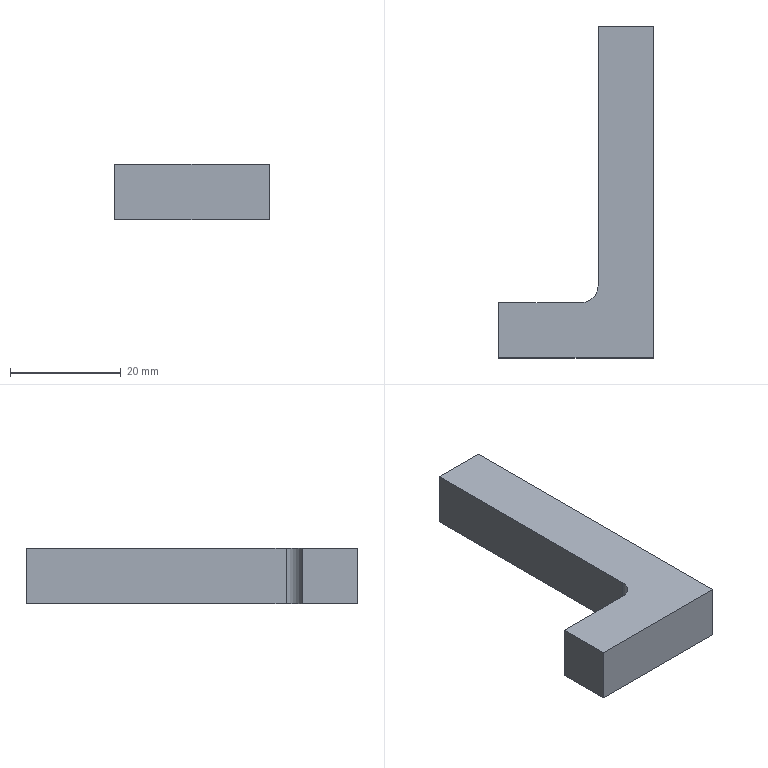Part | STEP file | 001-003-Shaft storage support plate reinforcing rib | 1 solid | 9 faces | box 28 x 60 x 10 mm | volume 7819 mm3 | plane 8 | cylinder 1 | commonest cylinder face diameters 6 x1
STEP:
#1=CARTESIAN_POINT('',(0.,0.,0.));
#2=DIRECTION('',(0.,0.,1.));
#3=DIRECTION('',(1.,0.,0.));
#4=AXIS2_PLACEMENT_3D('',#1,#2,#3);
#5=CARTESIAN_POINT('',(14.,-30.,0.));
#6=VERTEX_POINT('',#5);
#7=CARTESIAN_POINT('',(14.,30.,0.));
#8=VERTEX_POINT('',#7);
#9=CARTESIAN_POINT('',(14.,-30.,0.));
#10=DIRECTION('',(0.,1.,0.));
#11=VECTOR('',#10,1.);
#12=LINE('',#9,#11);
#13=CARTESIAN_POINT('',(14.,-30.,10.));
#14=DIRECTION('',(-1.,0.,0.));
#15=DIRECTION('',(0.,0.,1.));
#16=AXIS2_PLACEMENT_3D('',#13,#14,#15);
#17=PLANE('',#16);
#18=CARTESIAN_POINT('',(-10.,0.));
#19=DIRECTION('',(0.,1.));
#20=VECTOR('',#19,1.);
#21=LINE('',#18,#20);
#22=(GEOMETRIC_REPRESENTATION_CONTEXT(2)PARAMETRIC_REPRESENTATION_CONTEXT()REPRESENTATION_CONTEXT('',''));
#23=DEFINITIONAL_REPRESENTATION('',(#21),#22);
#24=PCURVE('',#17,#23);
#25=CARTESIAN_POINT('',(0.,0.,0.));
#26=DIRECTION('',(0.,0.,-1.));
#27=DIRECTION('',(-1.,0.,0.));
#28=AXIS2_PLACEMENT_3D('',#25,#26,#27);
#29=PLANE('',#28);
#30=CARTESIAN_POINT('',(-14.,-30.));
#31=DIRECTION('',(0.,1.));
#32=VECTOR('',#31,1.);
#33=LINE('',#30,#32);
#34=(GEOMETRIC_REPRESENTATION_CONTEXT(2)PARAMETRIC_REPRESENTATION_CONTEXT()REPRESENTATION_CONTEXT('',''));
#35=DEFINITIONAL_REPRESENTATION('',(#33),#34);
#36=PCURVE('',#29,#35);
#37=SURFACE_CURVE('',#12,(#24,#36),.PCURVE_S1.);
#38=EDGE_CURVE('',#6,#8,#37,.T.);
#39=ORIENTED_EDGE('',*,*,#38,.T.);
#40=CARTESIAN_POINT('',(14.,30.,10.));
#41=VERTEX_POINT('',#40);
#42=CARTESIAN_POINT('',(14.,30.,10.));
#43=DIRECTION('',(0.,0.,-1.));
#44=VECTOR('',#43,1.);
#45=LINE('',#42,#44);
#46=CARTESIAN_POINT('',(0.,60.));
#47=DIRECTION('',(-1.,0.));
#48=VECTOR('',#47,1.);
#49=LINE('',#46,#48);
#50=(GEOMETRIC_REPRESENTATION_CONTEXT(2)PARAMETRIC_REPRESENTATION_CONTEXT()REPRESENTATION_CONTEXT('',''));
#51=DEFINITIONAL_REPRESENTATION('',(#49),#50);
#52=PCURVE('',#17,#51);
#53=CARTESIAN_POINT('',(-14.,30.,10.));
#54=DIRECTION('',(0.,-1.,0.));
#55=DIRECTION('',(0.,0.,-1.));
#56=AXIS2_PLACEMENT_3D('',#53,#54,#55);
#57=PLANE('',#56);
#58=CARTESIAN_POINT('',(0.,28.));
#59=DIRECTION('',(1.,0.));
#60=VECTOR('',#59,1.);
#61=LINE('',#58,#60);
#62=(GEOMETRIC_REPRESENTATION_CONTEXT(2)PARAMETRIC_REPRESENTATION_CONTEXT()REPRESENTATION_CONTEXT('',''));
#63=DEFINITIONAL_REPRESENTATION('',(#61),#62);
#64=PCURVE('',#57,#63);
#65=SURFACE_CURVE('',#45,(#52,#64),.PCURVE_S1.);
#66=EDGE_CURVE('',#41,#8,#65,.T.);
#67=ORIENTED_EDGE('',*,*,#66,.F.);
#68=CARTESIAN_POINT('',(14.,-30.,10.));
#69=VERTEX_POINT('',#68);
#70=CARTESIAN_POINT('',(14.,-30.,10.));
#71=DIRECTION('',(0.,1.,0.));
#72=VECTOR('',#71,1.);
#73=LINE('',#70,#72);
#74=CARTESIAN_POINT('',(0.,0.));
#75=DIRECTION('',(0.,1.));
#76=VECTOR('',#75,1.);
#77=LINE('',#74,#76);
#78=(GEOMETRIC_REPRESENTATION_CONTEXT(2)PARAMETRIC_REPRESENTATION_CONTEXT()REPRESENTATION_CONTEXT('',''));
#79=DEFINITIONAL_REPRESENTATION('',(#77),#78);
#80=PCURVE('',#17,#79);
#81=CARTESIAN_POINT('',(0.,0.,10.));
#82=DIRECTION('',(0.,0.,-1.));
#83=DIRECTION('',(-1.,0.,0.));
#84=AXIS2_PLACEMENT_3D('',#81,#82,#83);
#85=PLANE('',#84);
#86=CARTESIAN_POINT('',(-14.,-30.));
#87=DIRECTION('',(0.,1.));
#88=VECTOR('',#87,1.);
#89=LINE('',#86,#88);
#90=(GEOMETRIC_REPRESENTATION_CONTEXT(2)PARAMETRIC_REPRESENTATION_CONTEXT()REPRESENTATION_CONTEXT('',''));
#91=DEFINITIONAL_REPRESENTATION('',(#89),#90);
#92=PCURVE('',#85,#91);
#93=SURFACE_CURVE('',#73,(#80,#92),.PCURVE_S1.);
#94=EDGE_CURVE('',#69,#41,#93,.T.);
#95=ORIENTED_EDGE('',*,*,#94,.F.);
#96=CARTESIAN_POINT('',(14.,-30.,10.));
#97=DIRECTION('',(0.,0.,-1.));
#98=VECTOR('',#97,1.);
#99=LINE('',#96,#98);
#100=CARTESIAN_POINT('',(0.,0.));
#101=DIRECTION('',(-1.,0.));
#102=VECTOR('',#101,1.);
#103=LINE('',#100,#102);
#104=(GEOMETRIC_REPRESENTATION_CONTEXT(2)PARAMETRIC_REPRESENTATION_CONTEXT()REPRESENTATION_CONTEXT('',''));
#105=DEFINITIONAL_REPRESENTATION('',(#103),#104);
#106=PCURVE('',#17,#105);
#107=CARTESIAN_POINT('',(-14.,-30.,10.));
#108=DIRECTION('',(0.,1.,0.));
#109=DIRECTION('',(0.,0.,1.));
#110=AXIS2_PLACEMENT_3D('',#107,#108,#109);
#111=PLANE('',#110);
#112=CARTESIAN_POINT('',(0.,28.));
#113=DIRECTION('',(-1.,0.));
#114=VECTOR('',#113,1.);
#115=LINE('',#112,#114);
#116=(GEOMETRIC_REPRESENTATION_CONTEXT(2)PARAMETRIC_REPRESENTATION_CONTEXT()REPRESENTATION_CONTEXT('',''));
#117=DEFINITIONAL_REPRESENTATION('',(#115),#116);
#118=PCURVE('',#111,#117);
#119=SURFACE_CURVE('',#99,(#106,#118),.PCURVE_S1.);
#120=EDGE_CURVE('',#69,#6,#119,.T.);
#121=ORIENTED_EDGE('',*,*,#120,.T.);
#122=EDGE_LOOP('',(#39,#67,#95,#121));
#123=FACE_BOUND('',#122,.T.);
#124=ADVANCED_FACE('',(#123),#17,.F.);
#125=CARTESIAN_POINT('',(4.,30.,0.));
#126=VERTEX_POINT('',#125);
#127=CARTESIAN_POINT('',(-14.,30.,0.));
#128=DIRECTION('',(-1.,0.,0.));
#129=VECTOR('',#128,1.);
#130=LINE('',#127,#129);
#131=CARTESIAN_POINT('',(10.,0.));
#132=DIRECTION('',(0.,-1.));
#133=VECTOR('',#132,1.);
#134=LINE('',#131,#133);
#135=(GEOMETRIC_REPRESENTATION_CONTEXT(2)PARAMETRIC_REPRESENTATION_CONTEXT()REPRESENTATION_CONTEXT('',''));
#136=DEFINITIONAL_REPRESENTATION('',(#134),#135);
#137=PCURVE('',#57,#136);
#138=CARTESIAN_POINT('',(14.,30.));
#139=DIRECTION('',(1.,0.));
#140=VECTOR('',#139,1.);
#141=LINE('',#138,#140);
#142=(GEOMETRIC_REPRESENTATION_CONTEXT(2)PARAMETRIC_REPRESENTATION_CONTEXT()REPRESENTATION_CONTEXT('',''));
#143=DEFINITIONAL_REPRESENTATION('',(#141),#142);
#144=PCURVE('',#29,#143);
#145=SURFACE_CURVE('',#130,(#137,#144),.PCURVE_S1.);
#146=EDGE_CURVE('',#8,#126,#145,.T.);
#147=ORIENTED_EDGE('',*,*,#146,.T.);
#148=CARTESIAN_POINT('',(4.,30.,10.));
#149=VERTEX_POINT('',#148);
#150=CARTESIAN_POINT('',(4.,30.,0.));
#151=DIRECTION('',(0.,0.,1.));
#152=VECTOR('',#151,1.);
#153=LINE('',#150,#152);
#154=CARTESIAN_POINT('',(10.,18.));
#155=DIRECTION('',(-1.,0.));
#156=VECTOR('',#155,1.);
#157=LINE('',#154,#156);
#158=(GEOMETRIC_REPRESENTATION_CONTEXT(2)PARAMETRIC_REPRESENTATION_CONTEXT()REPRESENTATION_CONTEXT('',''));
#159=DEFINITIONAL_REPRESENTATION('',(#157),#158);
#160=PCURVE('',#57,#159);
#161=CARTESIAN_POINT('',(4.,30.,0.));
#162=DIRECTION('',(1.,0.,0.));
#163=DIRECTION('',(0.,1.,0.));
#164=AXIS2_PLACEMENT_3D('',#161,#162,#163);
#165=PLANE('',#164);
#166=CARTESIAN_POINT('',(0.,0.));
#167=DIRECTION('',(0.,1.));
#168=VECTOR('',#167,1.);
#169=LINE('',#166,#168);
#170=(GEOMETRIC_REPRESENTATION_CONTEXT(2)PARAMETRIC_REPRESENTATION_CONTEXT()REPRESENTATION_CONTEXT('',''));
#171=DEFINITIONAL_REPRESENTATION('',(#169),#170);
#172=PCURVE('',#165,#171);
#173=SURFACE_CURVE('',#153,(#160,#172),.PCURVE_S1.);
#174=EDGE_CURVE('',#126,#149,#173,.T.);
#175=ORIENTED_EDGE('',*,*,#174,.T.);
#176=CARTESIAN_POINT('',(-14.,30.,10.));
#177=DIRECTION('',(-1.,0.,0.));
#178=VECTOR('',#177,1.);
#179=LINE('',#176,#178);
#180=CARTESIAN_POINT('',(0.,0.));
#181=DIRECTION('',(0.,-1.));
#182=VECTOR('',#181,1.);
#183=LINE('',#180,#182);
#184=(GEOMETRIC_REPRESENTATION_CONTEXT(2)PARAMETRIC_REPRESENTATION_CONTEXT()REPRESENTATION_CONTEXT('',''));
#185=DEFINITIONAL_REPRESENTATION('',(#183),#184);
#186=PCURVE('',#57,#185);
#187=CARTESIAN_POINT('',(14.,30.));
#188=DIRECTION('',(1.,0.));
#189=VECTOR('',#188,1.);
#190=LINE('',#187,#189);
#191=(GEOMETRIC_REPRESENTATION_CONTEXT(2)PARAMETRIC_REPRESENTATION_CONTEXT()REPRESENTATION_CONTEXT('',''));
#192=DEFINITIONAL_REPRESENTATION('',(#190),#191);
#193=PCURVE('',#85,#192);
#194=SURFACE_CURVE('',#179,(#186,#193),.PCURVE_S1.);
#195=EDGE_CURVE('',#41,#149,#194,.T.);
#196=ORIENTED_EDGE('',*,*,#195,.F.);
#197=ORIENTED_EDGE('',*,*,#66,.T.);
#198=EDGE_LOOP('',(#147,#175,#196,#197));
#199=FACE_BOUND('',#198,.T.);
#200=ADVANCED_FACE('',(#199),#57,.F.);
#201=CARTESIAN_POINT('',(-14.,-20.,10.));
#202=VERTEX_POINT('',#201);
#203=CARTESIAN_POINT('',(-14.,-30.,10.));
#204=VERTEX_POINT('',#203);
#205=CARTESIAN_POINT('',(-14.,-30.,10.));
#206=DIRECTION('',(0.,-1.,0.));
#207=VECTOR('',#206,1.);
#208=LINE('',#205,#207);
#209=CARTESIAN_POINT('',(-14.,-30.,10.));
#210=DIRECTION('',(1.,0.,0.));
#211=DIRECTION('',(0.,0.,-1.));
#212=AXIS2_PLACEMENT_3D('',#209,#210,#211);
#213=PLANE('',#212);
#214=CARTESIAN_POINT('',(0.,0.));
#215=DIRECTION('',(0.,-1.));
#216=VECTOR('',#215,1.);
#217=LINE('',#214,#216);
#218=(GEOMETRIC_REPRESENTATION_CONTEXT(2)PARAMETRIC_REPRESENTATION_CONTEXT()REPRESENTATION_CONTEXT('',''));
#219=DEFINITIONAL_REPRESENTATION('',(#217),#218);
#220=PCURVE('',#213,#219);
#221=CARTESIAN_POINT('',(14.,-30.));
#222=DIRECTION('',(0.,-1.));
#223=VECTOR('',#222,1.);
#224=LINE('',#221,#223);
#225=(GEOMETRIC_REPRESENTATION_CONTEXT(2)PARAMETRIC_REPRESENTATION_CONTEXT()REPRESENTATION_CONTEXT('',''));
#226=DEFINITIONAL_REPRESENTATION('',(#224),#225);
#227=PCURVE('',#85,#226);
#228=SURFACE_CURVE('',#208,(#220,#227),.PCURVE_S1.);
#229=EDGE_CURVE('',#202,#204,#228,.T.);
#230=ORIENTED_EDGE('',*,*,#229,.F.);
#231=CARTESIAN_POINT('',(-14.,-20.,0.));
#232=VERTEX_POINT('',#231);
#233=CARTESIAN_POINT('',(-14.,-20.,0.));
#234=DIRECTION('',(0.,0.,1.));
#235=VECTOR('',#234,1.);
#236=LINE('',#233,#235);
#237=CARTESIAN_POINT('',(10.,10.));
#238=DIRECTION('',(-1.,0.));
#239=VECTOR('',#238,1.);
#240=LINE('',#237,#239);
#241=(GEOMETRIC_REPRESENTATION_CONTEXT(2)PARAMETRIC_REPRESENTATION_CONTEXT()REPRESENTATION_CONTEXT('',''));
#242=DEFINITIONAL_REPRESENTATION('',(#240),#241);
#243=PCURVE('',#213,#242);
#244=CARTESIAN_POINT('',(-14.,-20.,0.));
#245=DIRECTION('',(0.,-1.,0.));
#246=DIRECTION('',(1.,0.,0.));
#247=AXIS2_PLACEMENT_3D('',#244,#245,#246);
#248=PLANE('',#247);
#249=CARTESIAN_POINT('',(0.,0.));
#250=DIRECTION('',(0.,1.));
#251=VECTOR('',#250,1.);
#252=LINE('',#249,#251);
#253=(GEOMETRIC_REPRESENTATION_CONTEXT(2)PARAMETRIC_REPRESENTATION_CONTEXT()REPRESENTATION_CONTEXT('',''));
#254=DEFINITIONAL_REPRESENTATION('',(#252),#253);
#255=PCURVE('',#248,#254);
#256=SURFACE_CURVE('',#236,(#243,#255),.PCURVE_S1.);
#257=EDGE_CURVE('',#232,#202,#256,.T.);
#258=ORIENTED_EDGE('',*,*,#257,.F.);
#259=CARTESIAN_POINT('',(-14.,-30.,0.));
#260=VERTEX_POINT('',#259);
#261=CARTESIAN_POINT('',(-14.,-30.,0.));
#262=DIRECTION('',(0.,-1.,0.));
#263=VECTOR('',#262,1.);
#264=LINE('',#261,#263);
#265=CARTESIAN_POINT('',(10.,0.));
#266=DIRECTION('',(0.,-1.));
#267=VECTOR('',#266,1.);
#268=LINE('',#265,#267);
#269=(GEOMETRIC_REPRESENTATION_CONTEXT(2)PARAMETRIC_REPRESENTATION_CONTEXT()REPRESENTATION_CONTEXT('',''));
#270=DEFINITIONAL_REPRESENTATION('',(#268),#269);
#271=PCURVE('',#213,#270);
#272=CARTESIAN_POINT('',(14.,-30.));
#273=DIRECTION('',(0.,-1.));
#274=VECTOR('',#273,1.);
#275=LINE('',#272,#274);
#276=(GEOMETRIC_REPRESENTATION_CONTEXT(2)PARAMETRIC_REPRESENTATION_CONTEXT()REPRESENTATION_CONTEXT('',''));
#277=DEFINITIONAL_REPRESENTATION('',(#275),#276);
#278=PCURVE('',#29,#277);
#279=SURFACE_CURVE('',#264,(#271,#278),.PCURVE_S1.);
#280=EDGE_CURVE('',#232,#260,#279,.T.);
#281=ORIENTED_EDGE('',*,*,#280,.T.);
#282=CARTESIAN_POINT('',(-14.,-30.,10.));
#283=DIRECTION('',(0.,0.,-1.));
#284=VECTOR('',#283,1.);
#285=LINE('',#282,#284);
#286=CARTESIAN_POINT('',(0.,0.));
#287=DIRECTION('',(1.,0.));
#288=VECTOR('',#287,1.);
#289=LINE('',#286,#288);
#290=(GEOMETRIC_REPRESENTATION_CONTEXT(2)PARAMETRIC_REPRESENTATION_CONTEXT()REPRESENTATION_CONTEXT('',''));
#291=DEFINITIONAL_REPRESENTATION('',(#289),#290);
#292=PCURVE('',#213,#291);
#293=CARTESIAN_POINT('',(0.,0.));
#294=DIRECTION('',(-1.,0.));
#295=VECTOR('',#294,1.);
#296=LINE('',#293,#295);
#297=(GEOMETRIC_REPRESENTATION_CONTEXT(2)PARAMETRIC_REPRESENTATION_CONTEXT()REPRESENTATION_CONTEXT('',''));
#298=DEFINITIONAL_REPRESENTATION('',(#296),#297);
#299=PCURVE('',#111,#298);
#300=SURFACE_CURVE('',#285,(#292,#299),.PCURVE_S1.);
#301=EDGE_CURVE('',#204,#260,#300,.T.);
#302=ORIENTED_EDGE('',*,*,#301,.F.);
#303=EDGE_LOOP('',(#230,#258,#281,#302));
#304=FACE_BOUND('',#303,.T.);
#305=ADVANCED_FACE('',(#304),#213,.F.);
#306=CARTESIAN_POINT('',(-14.,-30.,0.));
#307=DIRECTION('',(1.,0.,0.));
#308=VECTOR('',#307,1.);
#309=LINE('',#306,#308);
#310=CARTESIAN_POINT('',(-10.,0.));
#311=DIRECTION('',(0.,1.));
#312=VECTOR('',#311,1.);
#313=LINE('',#310,#312);
#314=(GEOMETRIC_REPRESENTATION_CONTEXT(2)PARAMETRIC_REPRESENTATION_CONTEXT()REPRESENTATION_CONTEXT('',''));
#315=DEFINITIONAL_REPRESENTATION('',(#313),#314);
#316=PCURVE('',#111,#315);
#317=CARTESIAN_POINT('',(14.,-30.));
#318=DIRECTION('',(-1.,0.));
#319=VECTOR('',#318,1.);
#320=LINE('',#317,#319);
#321=(GEOMETRIC_REPRESENTATION_CONTEXT(2)PARAMETRIC_REPRESENTATION_CONTEXT()REPRESENTATION_CONTEXT('',''));
#322=DEFINITIONAL_REPRESENTATION('',(#320),#321);
#323=PCURVE('',#29,#322);
#324=SURFACE_CURVE('',#309,(#316,#323),.PCURVE_S1.);
#325=EDGE_CURVE('',#260,#6,#324,.T.);
#326=ORIENTED_EDGE('',*,*,#325,.T.);
#327=ORIENTED_EDGE('',*,*,#120,.F.);
#328=CARTESIAN_POINT('',(-14.,-30.,10.));
#329=DIRECTION('',(1.,0.,0.));
#330=VECTOR('',#329,1.);
#331=LINE('',#328,#330);
#332=CARTESIAN_POINT('',(0.,0.));
#333=DIRECTION('',(0.,1.));
#334=VECTOR('',#333,1.);
#335=LINE('',#332,#334);
#336=(GEOMETRIC_REPRESENTATION_CONTEXT(2)PARAMETRIC_REPRESENTATION_CONTEXT()REPRESENTATION_CONTEXT('',''));
#337=DEFINITIONAL_REPRESENTATION('',(#335),#336);
#338=PCURVE('',#111,#337);
#339=CARTESIAN_POINT('',(14.,-30.));
#340=DIRECTION('',(-1.,0.));
#341=VECTOR('',#340,1.);
#342=LINE('',#339,#341);
#343=(GEOMETRIC_REPRESENTATION_CONTEXT(2)PARAMETRIC_REPRESENTATION_CONTEXT()REPRESENTATION_CONTEXT('',''));
#344=DEFINITIONAL_REPRESENTATION('',(#342),#343);
#345=PCURVE('',#85,#344);
#346=SURFACE_CURVE('',#331,(#338,#345),.PCURVE_S1.);
#347=EDGE_CURVE('',#204,#69,#346,.T.);
#348=ORIENTED_EDGE('',*,*,#347,.F.);
#349=ORIENTED_EDGE('',*,*,#301,.T.);
#350=EDGE_LOOP('',(#326,#327,#348,#349));
#351=FACE_BOUND('',#350,.T.);
#352=ADVANCED_FACE('',(#351),#111,.F.);
#353=ORIENTED_EDGE('',*,*,#195,.T.);
#354=CARTESIAN_POINT('',(4.,-17.,10.));
#355=VERTEX_POINT('',#354);
#356=CARTESIAN_POINT('',(4.,30.,10.));
#357=DIRECTION('',(0.,1.,0.));
#358=VECTOR('',#357,1.);
#359=LINE('',#356,#358);
#360=CARTESIAN_POINT('',(-4.,30.));
#361=DIRECTION('',(0.,1.));
#362=VECTOR('',#361,1.);
#363=LINE('',#360,#362);
#364=(GEOMETRIC_REPRESENTATION_CONTEXT(2)PARAMETRIC_REPRESENTATION_CONTEXT()REPRESENTATION_CONTEXT('',''));
#365=DEFINITIONAL_REPRESENTATION('',(#363),#364);
#366=PCURVE('',#85,#365);
#367=CARTESIAN_POINT('',(0.,10.));
#368=DIRECTION('',(1.,0.));
#369=VECTOR('',#368,1.);
#370=LINE('',#367,#369);
#371=(GEOMETRIC_REPRESENTATION_CONTEXT(2)PARAMETRIC_REPRESENTATION_CONTEXT()REPRESENTATION_CONTEXT('',''));
#372=DEFINITIONAL_REPRESENTATION('',(#370),#371);
#373=PCURVE('',#165,#372);
#374=SURFACE_CURVE('',#359,(#366,#373),.PCURVE_S1.);
#375=EDGE_CURVE('',#355,#149,#374,.T.);
#376=ORIENTED_EDGE('',*,*,#375,.F.);
#377=CARTESIAN_POINT('',(1.,-20.,10.));
#378=VERTEX_POINT('',#377);
#379=CARTESIAN_POINT('',(1.,-17.,10.));
#380=DIRECTION('',(0.,0.,-1.));
#381=DIRECTION('',(-1.,0.,0.));
#382=AXIS2_PLACEMENT_3D('',#379,#380,#381);
#383=CIRCLE('',#382,3.);
#384=CARTESIAN_POINT('',(-1.,-17.));
#385=DIRECTION('',(1.,0.));
#386=AXIS2_PLACEMENT_2D('',#384,#385);
#387=CIRCLE('',#386,3.);
#388=(GEOMETRIC_REPRESENTATION_CONTEXT(2)PARAMETRIC_REPRESENTATION_CONTEXT()REPRESENTATION_CONTEXT('',''));
#389=DEFINITIONAL_REPRESENTATION('',(#387),#388);
#390=PCURVE('',#85,#389);
#391=CARTESIAN_POINT('',(1.,-17.,0.));
#392=DIRECTION('',(0.,0.,-1.));
#393=DIRECTION('',(-1.,0.,0.));
#394=AXIS2_PLACEMENT_3D('',#391,#392,#393);
#395=CYLINDRICAL_SURFACE('',#394,3.);
#396=CARTESIAN_POINT('',(0.,-10.));
#397=DIRECTION('',(1.,0.));
#398=VECTOR('',#397,1.);
#399=LINE('',#396,#398);
#400=(GEOMETRIC_REPRESENTATION_CONTEXT(2)PARAMETRIC_REPRESENTATION_CONTEXT()REPRESENTATION_CONTEXT('',''));
#401=DEFINITIONAL_REPRESENTATION('',(#399),#400);
#402=PCURVE('',#395,#401);
#403=SURFACE_CURVE('',#383,(#390,#402),.PCURVE_S1.);
#404=EDGE_CURVE('',#355,#378,#403,.T.);
#405=ORIENTED_EDGE('',*,*,#404,.T.);
#406=CARTESIAN_POINT('',(-14.,-20.,10.));
#407=DIRECTION('',(1.,0.,0.));
#408=VECTOR('',#407,1.);
#409=LINE('',#406,#408);
#410=CARTESIAN_POINT('',(14.,-20.));
#411=DIRECTION('',(-1.,0.));
#412=VECTOR('',#411,1.);
#413=LINE('',#410,#412);
#414=(GEOMETRIC_REPRESENTATION_CONTEXT(2)PARAMETRIC_REPRESENTATION_CONTEXT()REPRESENTATION_CONTEXT('',''));
#415=DEFINITIONAL_REPRESENTATION('',(#413),#414);
#416=PCURVE('',#85,#415);
#417=CARTESIAN_POINT('',(0.,10.));
#418=DIRECTION('',(1.,0.));
#419=VECTOR('',#418,1.);
#420=LINE('',#417,#419);
#421=(GEOMETRIC_REPRESENTATION_CONTEXT(2)PARAMETRIC_REPRESENTATION_CONTEXT()REPRESENTATION_CONTEXT('',''));
#422=DEFINITIONAL_REPRESENTATION('',(#420),#421);
#423=PCURVE('',#248,#422);
#424=SURFACE_CURVE('',#409,(#416,#423),.PCURVE_S1.);
#425=EDGE_CURVE('',#202,#378,#424,.T.);
#426=ORIENTED_EDGE('',*,*,#425,.F.);
#427=ORIENTED_EDGE('',*,*,#229,.T.);
#428=ORIENTED_EDGE('',*,*,#347,.T.);
#429=ORIENTED_EDGE('',*,*,#94,.T.);
#430=EDGE_LOOP('',(#353,#376,#405,#426,#427,#428,#429));
#431=FACE_BOUND('',#430,.T.);
#432=ADVANCED_FACE('',(#431),#85,.F.);
#433=CARTESIAN_POINT('',(1.,-20.,0.));
#434=VERTEX_POINT('',#433);
#435=CARTESIAN_POINT('',(-14.,-20.,0.));
#436=DIRECTION('',(1.,0.,0.));
#437=VECTOR('',#436,1.);
#438=LINE('',#435,#437);
#439=CARTESIAN_POINT('',(14.,-20.));
#440=DIRECTION('',(-1.,0.));
#441=VECTOR('',#440,1.);
#442=LINE('',#439,#441);
#443=(GEOMETRIC_REPRESENTATION_CONTEXT(2)PARAMETRIC_REPRESENTATION_CONTEXT()REPRESENTATION_CONTEXT('',''));
#444=DEFINITIONAL_REPRESENTATION('',(#442),#443);
#445=PCURVE('',#29,#444);
#446=CARTESIAN_POINT('',(0.,0.));
#447=DIRECTION('',(1.,0.));
#448=VECTOR('',#447,1.);
#449=LINE('',#446,#448);
#450=(GEOMETRIC_REPRESENTATION_CONTEXT(2)PARAMETRIC_REPRESENTATION_CONTEXT()REPRESENTATION_CONTEXT('',''));
#451=DEFINITIONAL_REPRESENTATION('',(#449),#450);
#452=PCURVE('',#248,#451);
#453=SURFACE_CURVE('',#438,(#445,#452),.PCURVE_S1.);
#454=EDGE_CURVE('',#232,#434,#453,.T.);
#455=ORIENTED_EDGE('',*,*,#454,.T.);
#456=CARTESIAN_POINT('',(4.,-17.,0.));
#457=VERTEX_POINT('',#456);
#458=CARTESIAN_POINT('',(1.,-17.,0.));
#459=DIRECTION('',(0.,0.,1.));
#460=DIRECTION('',(-1.,0.,0.));
#461=AXIS2_PLACEMENT_3D('',#458,#459,#460);
#462=CIRCLE('',#461,3.);
#463=CARTESIAN_POINT('',(2.,-17.));
#464=CARTESIAN_POINT('',(2.,-22.196));
#465=CARTESIAN_POINT('',(-2.5,-19.598));
#466=CARTESIAN_POINT('',(-7.,-17.));
#467=CARTESIAN_POINT('',(-2.5,-14.402));
#468=CARTESIAN_POINT('',(2.,-11.804));
#469=CARTESIAN_POINT('',(2.,-17.));
#470=(BOUNDED_CURVE()B_SPLINE_CURVE(2,(#463,#464,#465,#466,#467,#468,#469),.UNSPECIFIED.,.T.,.F.)B_SPLINE_CURVE_WITH_KNOTS((1,2,2,2,2,1),(-2.094,0.,2.094,4.189,6.283,8.378),.UNSPECIFIED.)CURVE()GEOMETRIC_REPRESENTATION_ITEM()RATIONAL_B_SPLINE_CURVE((1.,0.5,1.,0.5,1.,0.5,1.))REPRESENTATION_ITEM(''));
#471=(GEOMETRIC_REPRESENTATION_CONTEXT(2)PARAMETRIC_REPRESENTATION_CONTEXT()REPRESENTATION_CONTEXT('',''));
#472=DEFINITIONAL_REPRESENTATION('',(#470),#471);
#473=PCURVE('',#29,#472);
#474=CARTESIAN_POINT('',(6.283,0.));
#475=DIRECTION('',(-1.,0.));
#476=VECTOR('',#475,1.);
#477=LINE('',#474,#476);
#478=(GEOMETRIC_REPRESENTATION_CONTEXT(2)PARAMETRIC_REPRESENTATION_CONTEXT()REPRESENTATION_CONTEXT('',''));
#479=DEFINITIONAL_REPRESENTATION('',(#477),#478);
#480=PCURVE('',#395,#479);
#481=SURFACE_CURVE('',#462,(#473,#480),.PCURVE_S1.);
#482=EDGE_CURVE('',#434,#457,#481,.T.);
#483=ORIENTED_EDGE('',*,*,#482,.T.);
#484=CARTESIAN_POINT('',(4.,30.,0.));
#485=DIRECTION('',(0.,1.,0.));
#486=VECTOR('',#485,1.);
#487=LINE('',#484,#486);
#488=CARTESIAN_POINT('',(-4.,30.));
#489=DIRECTION('',(0.,1.));
#490=VECTOR('',#489,1.);
#491=LINE('',#488,#490);
#492=(GEOMETRIC_REPRESENTATION_CONTEXT(2)PARAMETRIC_REPRESENTATION_CONTEXT()REPRESENTATION_CONTEXT('',''));
#493=DEFINITIONAL_REPRESENTATION('',(#491),#492);
#494=PCURVE('',#29,#493);
#495=CARTESIAN_POINT('',(0.,0.));
#496=DIRECTION('',(1.,0.));
#497=VECTOR('',#496,1.);
#498=LINE('',#495,#497);
#499=(GEOMETRIC_REPRESENTATION_CONTEXT(2)PARAMETRIC_REPRESENTATION_CONTEXT()REPRESENTATION_CONTEXT('',''));
#500=DEFINITIONAL_REPRESENTATION('',(#498),#499);
#501=PCURVE('',#165,#500);
#502=SURFACE_CURVE('',#487,(#494,#501),.PCURVE_S1.);
#503=EDGE_CURVE('',#457,#126,#502,.T.);
#504=ORIENTED_EDGE('',*,*,#503,.T.);
#505=ORIENTED_EDGE('',*,*,#146,.F.);
#506=ORIENTED_EDGE('',*,*,#38,.F.);
#507=ORIENTED_EDGE('',*,*,#325,.F.);
#508=ORIENTED_EDGE('',*,*,#280,.F.);
#509=EDGE_LOOP('',(#455,#483,#504,#505,#506,#507,#508));
#510=FACE_BOUND('',#509,.T.);
#511=ADVANCED_FACE('',(#510),#29,.T.);
#512=ORIENTED_EDGE('',*,*,#503,.F.);
#513=CARTESIAN_POINT('',(4.,-17.,10.));
#514=DIRECTION('',(0.,0.,1.));
#515=VECTOR('',#514,1.);
#516=LINE('',#513,#515);
#517=CARTESIAN_POINT('',(-47.,10.));
#518=DIRECTION('',(0.,1.));
#519=VECTOR('',#518,1.);
#520=LINE('',#517,#519);
#521=(GEOMETRIC_REPRESENTATION_CONTEXT(2)PARAMETRIC_REPRESENTATION_CONTEXT()REPRESENTATION_CONTEXT('',''));
#522=DEFINITIONAL_REPRESENTATION('',(#520),#521);
#523=PCURVE('',#165,#522);
#524=CARTESIAN_POINT('',(3.142,-10.));
#525=DIRECTION('',(0.,-1.));
#526=VECTOR('',#525,1.);
#527=LINE('',#524,#526);
#528=(GEOMETRIC_REPRESENTATION_CONTEXT(2)PARAMETRIC_REPRESENTATION_CONTEXT()REPRESENTATION_CONTEXT('',''));
#529=DEFINITIONAL_REPRESENTATION('',(#527),#528);
#530=PCURVE('',#395,#529);
#531=SURFACE_CURVE('',#516,(#523,#530),.PCURVE_S1.);
#532=EDGE_CURVE('',#457,#355,#531,.T.);
#533=ORIENTED_EDGE('',*,*,#532,.T.);
#534=ORIENTED_EDGE('',*,*,#375,.T.);
#535=ORIENTED_EDGE('',*,*,#174,.F.);
#536=EDGE_LOOP('',(#512,#533,#534,#535));
#537=FACE_BOUND('',#536,.T.);
#538=ADVANCED_FACE('',(#537),#165,.F.);
#539=ORIENTED_EDGE('',*,*,#425,.T.);
#540=CARTESIAN_POINT('',(1.,-20.,0.));
#541=DIRECTION('',(0.,0.,-1.));
#542=VECTOR('',#541,1.);
#543=LINE('',#540,#542);
#544=CARTESIAN_POINT('',(15.,0.));
#545=DIRECTION('',(0.,-1.));
#546=VECTOR('',#545,1.);
#547=LINE('',#544,#546);
#548=(GEOMETRIC_REPRESENTATION_CONTEXT(2)PARAMETRIC_REPRESENTATION_CONTEXT()REPRESENTATION_CONTEXT('',''));
#549=DEFINITIONAL_REPRESENTATION('',(#547),#548);
#550=PCURVE('',#248,#549);
#551=CARTESIAN_POINT('',(4.712,0.));
#552=DIRECTION('',(0.,1.));
#553=VECTOR('',#552,1.);
#554=LINE('',#551,#553);
#555=(GEOMETRIC_REPRESENTATION_CONTEXT(2)PARAMETRIC_REPRESENTATION_CONTEXT()REPRESENTATION_CONTEXT('',''));
#556=DEFINITIONAL_REPRESENTATION('',(#554),#555);
#557=PCURVE('',#395,#556);
#558=SURFACE_CURVE('',#543,(#550,#557),.PCURVE_S1.);
#559=EDGE_CURVE('',#378,#434,#558,.T.);
#560=ORIENTED_EDGE('',*,*,#559,.T.);
#561=ORIENTED_EDGE('',*,*,#454,.F.);
#562=ORIENTED_EDGE('',*,*,#257,.T.);
#563=EDGE_LOOP('',(#539,#560,#561,#562));
#564=FACE_BOUND('',#563,.T.);
#565=ADVANCED_FACE('',(#564),#248,.F.);
#566=ORIENTED_EDGE('',*,*,#532,.T.);
#567=ORIENTED_EDGE('',*,*,#404,.T.);
#568=ORIENTED_EDGE('',*,*,#559,.T.);
#569=ORIENTED_EDGE('',*,*,#482,.T.);
#570=EDGE_LOOP('',(#566,#567,#568,#569));
#571=FACE_BOUND('',#570,.F.);
#572=ADVANCED_FACE('',(#571),#395,.F.);
#573=CLOSED_SHELL('',(#124,#200,#305,#352,#432,#511,#538,#565,#572));
#574=MANIFOLD_SOLID_BREP('',#573);
#575=(LENGTH_UNIT()NAMED_UNIT(*)SI_UNIT(.MILLI.,.METRE.));
#576=UNCERTAINTY_MEASURE_WITH_UNIT(LENGTH_MEASURE(0.0000001),#575,'','');
#577=(NAMED_UNIT(*)PLANE_ANGLE_UNIT()SI_UNIT($,.RADIAN.));
#578=(NAMED_UNIT(*)SI_UNIT($,.STERADIAN.)SOLID_ANGLE_UNIT());
#579=(GEOMETRIC_REPRESENTATION_CONTEXT(3)GLOBAL_UNCERTAINTY_ASSIGNED_CONTEXT((#576))GLOBAL_UNIT_ASSIGNED_CONTEXT((#575,#577,#578))REPRESENTATION_CONTEXT('',''));
#580=ADVANCED_BREP_SHAPE_REPRESENTATION('',(#4,#574),#579);